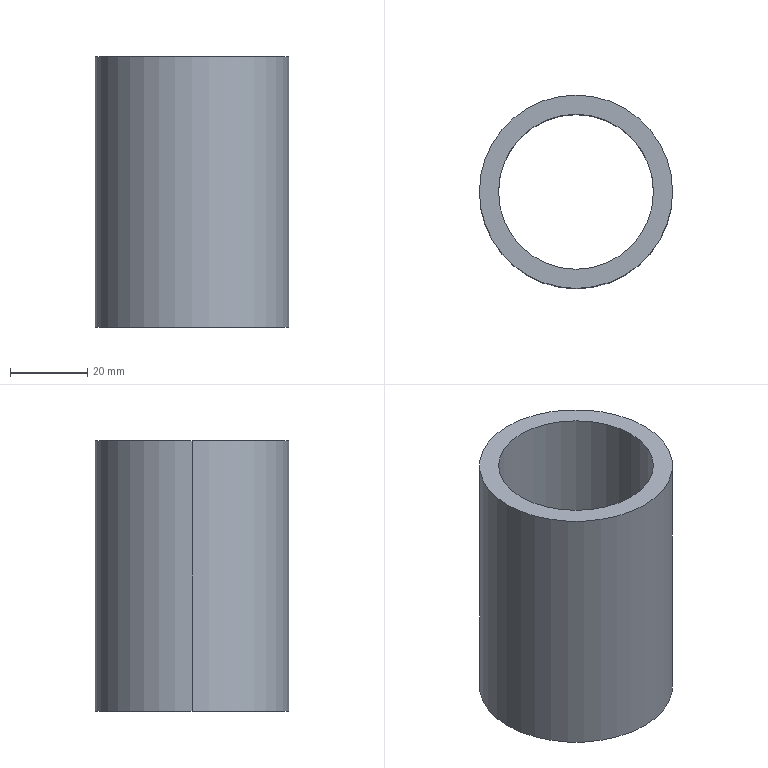Part | STEP file | LM-05-1230_default | 1 solid | 6 faces | box 50 x 50 x 70 mm | volume 49040 mm3 | cylinder 4 | plane 2 | commonest cylinder face diameters 40.1 x2 50 x2
STEP:
#1=CARTESIAN_POINT('',(0.,0.,0.));
#2=DIRECTION('',(0.,0.,1.));
#3=DIRECTION('',(1.,0.,0.));
#4=AXIS2_PLACEMENT_3D('',#1,#2,#3);
#5=CARTESIAN_POINT('',(-20.05,0.,35.));
#6=VERTEX_POINT('',#5);
#7=CARTESIAN_POINT('',(-20.05,0.,-35.));
#8=VERTEX_POINT('',#7);
#9=CARTESIAN_POINT('',(-20.05,0.,35.));
#10=DIRECTION('',(0.,0.,-1.));
#11=VECTOR('',#10,1.);
#12=LINE('',#9,#11);
#13=CARTESIAN_POINT('',(0.,0.,35.));
#14=DIRECTION('',(0.,0.,-1.));
#15=DIRECTION('',(-1.,0.,0.));
#16=AXIS2_PLACEMENT_3D('',#13,#14,#15);
#17=CYLINDRICAL_SURFACE('',#16,20.05);
#18=CARTESIAN_POINT('',(6.283,0.));
#19=DIRECTION('',(0.,1.));
#20=VECTOR('',#19,1.);
#21=LINE('',#18,#20);
#22=(GEOMETRIC_REPRESENTATION_CONTEXT(2)PARAMETRIC_REPRESENTATION_CONTEXT()REPRESENTATION_CONTEXT('',''));
#23=DEFINITIONAL_REPRESENTATION('',(#21),#22);
#24=PCURVE('',#17,#23);
#25=CARTESIAN_POINT('',(0.,0.,35.));
#26=DIRECTION('',(0.,0.,-1.));
#27=DIRECTION('',(-1.,0.,0.));
#28=AXIS2_PLACEMENT_3D('',#25,#26,#27);
#29=CYLINDRICAL_SURFACE('',#28,20.05);
#30=CARTESIAN_POINT('',(0.,0.));
#31=DIRECTION('',(0.,1.));
#32=VECTOR('',#31,1.);
#33=LINE('',#30,#32);
#34=(GEOMETRIC_REPRESENTATION_CONTEXT(2)PARAMETRIC_REPRESENTATION_CONTEXT()REPRESENTATION_CONTEXT('',''));
#35=DEFINITIONAL_REPRESENTATION('',(#33),#34);
#36=PCURVE('',#29,#35);
#37=SURFACE_CURVE('',#12,(#24,#36),.PCURVE_S1.);
#38=EDGE_CURVE('',#6,#8,#37,.T.);
#39=ORIENTED_EDGE('',*,*,#38,.T.);
#40=CARTESIAN_POINT('',(20.05,0.,-35.));
#41=VERTEX_POINT('',#40);
#42=CARTESIAN_POINT('',(0.,0.,-35.));
#43=DIRECTION('',(0.,0.,1.));
#44=DIRECTION('',(1.,0.,0.));
#45=AXIS2_PLACEMENT_3D('',#42,#43,#44);
#46=CIRCLE('',#45,20.05);
#47=CARTESIAN_POINT('',(9.425,70.));
#48=DIRECTION('',(-1.,0.));
#49=VECTOR('',#48,1.);
#50=LINE('',#47,#49);
#51=(GEOMETRIC_REPRESENTATION_CONTEXT(2)PARAMETRIC_REPRESENTATION_CONTEXT()REPRESENTATION_CONTEXT('',''));
#52=DEFINITIONAL_REPRESENTATION('',(#50),#51);
#53=PCURVE('',#17,#52);
#54=CARTESIAN_POINT('',(0.,0.,-35.));
#55=DIRECTION('',(0.,0.,1.));
#56=DIRECTION('',(1.,0.,0.));
#57=AXIS2_PLACEMENT_3D('',#54,#55,#56);
#58=PLANE('',#57);
#59=CARTESIAN_POINT('',(0.,0.));
#60=DIRECTION('',(1.,0.));
#61=AXIS2_PLACEMENT_2D('',#59,#60);
#62=CIRCLE('',#61,20.05);
#63=(GEOMETRIC_REPRESENTATION_CONTEXT(2)PARAMETRIC_REPRESENTATION_CONTEXT()REPRESENTATION_CONTEXT('',''));
#64=DEFINITIONAL_REPRESENTATION('',(#62),#63);
#65=PCURVE('',#58,#64);
#66=SURFACE_CURVE('',#46,(#53,#65),.PCURVE_S1.);
#67=EDGE_CURVE('',#8,#41,#66,.T.);
#68=ORIENTED_EDGE('',*,*,#67,.T.);
#69=CARTESIAN_POINT('',(20.05,0.,35.));
#70=VERTEX_POINT('',#69);
#71=CARTESIAN_POINT('',(20.05,0.,35.));
#72=DIRECTION('',(0.,0.,-1.));
#73=VECTOR('',#72,1.);
#74=LINE('',#71,#73);
#75=CARTESIAN_POINT('',(3.142,0.));
#76=DIRECTION('',(0.,1.));
#77=VECTOR('',#76,1.);
#78=LINE('',#75,#77);
#79=(GEOMETRIC_REPRESENTATION_CONTEXT(2)PARAMETRIC_REPRESENTATION_CONTEXT()REPRESENTATION_CONTEXT('',''));
#80=DEFINITIONAL_REPRESENTATION('',(#78),#79);
#81=PCURVE('',#17,#80);
#82=CARTESIAN_POINT('',(3.142,0.));
#83=DIRECTION('',(0.,1.));
#84=VECTOR('',#83,1.);
#85=LINE('',#82,#84);
#86=(GEOMETRIC_REPRESENTATION_CONTEXT(2)PARAMETRIC_REPRESENTATION_CONTEXT()REPRESENTATION_CONTEXT('',''));
#87=DEFINITIONAL_REPRESENTATION('',(#85),#86);
#88=PCURVE('',#29,#87);
#89=SURFACE_CURVE('',#74,(#81,#88),.PCURVE_S1.);
#90=EDGE_CURVE('',#70,#41,#89,.T.);
#91=ORIENTED_EDGE('',*,*,#90,.F.);
#92=CARTESIAN_POINT('',(0.,0.,35.));
#93=DIRECTION('',(0.,0.,1.));
#94=DIRECTION('',(1.,0.,0.));
#95=AXIS2_PLACEMENT_3D('',#92,#93,#94);
#96=CIRCLE('',#95,20.05);
#97=CARTESIAN_POINT('',(9.425,0.));
#98=DIRECTION('',(-1.,0.));
#99=VECTOR('',#98,1.);
#100=LINE('',#97,#99);
#101=(GEOMETRIC_REPRESENTATION_CONTEXT(2)PARAMETRIC_REPRESENTATION_CONTEXT()REPRESENTATION_CONTEXT('',''));
#102=DEFINITIONAL_REPRESENTATION('',(#100),#101);
#103=PCURVE('',#17,#102);
#104=CARTESIAN_POINT('',(0.,0.,35.));
#105=DIRECTION('',(0.,0.,1.));
#106=DIRECTION('',(1.,0.,0.));
#107=AXIS2_PLACEMENT_3D('',#104,#105,#106);
#108=PLANE('',#107);
#109=CARTESIAN_POINT('',(0.,0.));
#110=DIRECTION('',(1.,0.));
#111=AXIS2_PLACEMENT_2D('',#109,#110);
#112=CIRCLE('',#111,20.05);
#113=(GEOMETRIC_REPRESENTATION_CONTEXT(2)PARAMETRIC_REPRESENTATION_CONTEXT()REPRESENTATION_CONTEXT('',''));
#114=DEFINITIONAL_REPRESENTATION('',(#112),#113);
#115=PCURVE('',#108,#114);
#116=SURFACE_CURVE('',#96,(#103,#115),.PCURVE_S1.);
#117=EDGE_CURVE('',#6,#70,#116,.T.);
#118=ORIENTED_EDGE('',*,*,#117,.F.);
#119=EDGE_LOOP('',(#39,#68,#91,#118));
#120=FACE_BOUND('',#119,.F.);
#121=ADVANCED_FACE('',(#120),#17,.F.);
#122=CARTESIAN_POINT('',(25.,0.,35.));
#123=VERTEX_POINT('',#122);
#124=CARTESIAN_POINT('',(-25.,0.,35.));
#125=VERTEX_POINT('',#124);
#126=CARTESIAN_POINT('',(0.,0.,35.));
#127=DIRECTION('',(0.,0.,1.));
#128=DIRECTION('',(1.,0.,0.));
#129=AXIS2_PLACEMENT_3D('',#126,#127,#128);
#130=CIRCLE('',#129,25.);
#131=CARTESIAN_POINT('',(0.,0.,35.));
#132=DIRECTION('',(0.,0.,-1.));
#133=DIRECTION('',(-1.,0.,0.));
#134=AXIS2_PLACEMENT_3D('',#131,#132,#133);
#135=CYLINDRICAL_SURFACE('',#134,25.);
#136=CARTESIAN_POINT('',(3.142,0.));
#137=DIRECTION('',(-1.,0.));
#138=VECTOR('',#137,1.);
#139=LINE('',#136,#138);
#140=(GEOMETRIC_REPRESENTATION_CONTEXT(2)PARAMETRIC_REPRESENTATION_CONTEXT()REPRESENTATION_CONTEXT('',''));
#141=DEFINITIONAL_REPRESENTATION('',(#139),#140);
#142=PCURVE('',#135,#141);
#143=CARTESIAN_POINT('',(0.,0.));
#144=DIRECTION('',(1.,0.));
#145=AXIS2_PLACEMENT_2D('',#143,#144);
#146=CIRCLE('',#145,25.);
#147=(GEOMETRIC_REPRESENTATION_CONTEXT(2)PARAMETRIC_REPRESENTATION_CONTEXT()REPRESENTATION_CONTEXT('',''));
#148=DEFINITIONAL_REPRESENTATION('',(#146),#147);
#149=PCURVE('',#108,#148);
#150=SURFACE_CURVE('',#130,(#142,#149),.PCURVE_S1.);
#151=EDGE_CURVE('',#123,#125,#150,.T.);
#152=ORIENTED_EDGE('',*,*,#151,.F.);
#153=CARTESIAN_POINT('',(25.,0.,-35.));
#154=VERTEX_POINT('',#153);
#155=CARTESIAN_POINT('',(25.,0.,35.));
#156=DIRECTION('',(0.,0.,-1.));
#157=VECTOR('',#156,1.);
#158=LINE('',#155,#157);
#159=CARTESIAN_POINT('',(3.142,0.));
#160=DIRECTION('',(0.,1.));
#161=VECTOR('',#160,1.);
#162=LINE('',#159,#161);
#163=(GEOMETRIC_REPRESENTATION_CONTEXT(2)PARAMETRIC_REPRESENTATION_CONTEXT()REPRESENTATION_CONTEXT('',''));
#164=DEFINITIONAL_REPRESENTATION('',(#162),#163);
#165=PCURVE('',#135,#164);
#166=CARTESIAN_POINT('',(0.,0.,35.));
#167=DIRECTION('',(0.,0.,-1.));
#168=DIRECTION('',(-1.,0.,0.));
#169=AXIS2_PLACEMENT_3D('',#166,#167,#168);
#170=CYLINDRICAL_SURFACE('',#169,25.);
#171=CARTESIAN_POINT('',(3.142,0.));
#172=DIRECTION('',(0.,1.));
#173=VECTOR('',#172,1.);
#174=LINE('',#171,#173);
#175=(GEOMETRIC_REPRESENTATION_CONTEXT(2)PARAMETRIC_REPRESENTATION_CONTEXT()REPRESENTATION_CONTEXT('',''));
#176=DEFINITIONAL_REPRESENTATION('',(#174),#175);
#177=PCURVE('',#170,#176);
#178=SURFACE_CURVE('',#158,(#165,#177),.PCURVE_S1.);
#179=EDGE_CURVE('',#123,#154,#178,.T.);
#180=ORIENTED_EDGE('',*,*,#179,.T.);
#181=CARTESIAN_POINT('',(-25.,0.,-35.));
#182=VERTEX_POINT('',#181);
#183=CARTESIAN_POINT('',(0.,0.,-35.));
#184=DIRECTION('',(0.,0.,1.));
#185=DIRECTION('',(1.,0.,0.));
#186=AXIS2_PLACEMENT_3D('',#183,#184,#185);
#187=CIRCLE('',#186,25.);
#188=CARTESIAN_POINT('',(3.142,70.));
#189=DIRECTION('',(-1.,0.));
#190=VECTOR('',#189,1.);
#191=LINE('',#188,#190);
#192=(GEOMETRIC_REPRESENTATION_CONTEXT(2)PARAMETRIC_REPRESENTATION_CONTEXT()REPRESENTATION_CONTEXT('',''));
#193=DEFINITIONAL_REPRESENTATION('',(#191),#192);
#194=PCURVE('',#135,#193);
#195=CARTESIAN_POINT('',(0.,0.));
#196=DIRECTION('',(1.,0.));
#197=AXIS2_PLACEMENT_2D('',#195,#196);
#198=CIRCLE('',#197,25.);
#199=(GEOMETRIC_REPRESENTATION_CONTEXT(2)PARAMETRIC_REPRESENTATION_CONTEXT()REPRESENTATION_CONTEXT('',''));
#200=DEFINITIONAL_REPRESENTATION('',(#198),#199);
#201=PCURVE('',#58,#200);
#202=SURFACE_CURVE('',#187,(#194,#201),.PCURVE_S1.);
#203=EDGE_CURVE('',#154,#182,#202,.T.);
#204=ORIENTED_EDGE('',*,*,#203,.T.);
#205=CARTESIAN_POINT('',(-25.,0.,35.));
#206=DIRECTION('',(0.,0.,-1.));
#207=VECTOR('',#206,1.);
#208=LINE('',#205,#207);
#209=CARTESIAN_POINT('',(0.,0.));
#210=DIRECTION('',(0.,1.));
#211=VECTOR('',#210,1.);
#212=LINE('',#209,#211);
#213=(GEOMETRIC_REPRESENTATION_CONTEXT(2)PARAMETRIC_REPRESENTATION_CONTEXT()REPRESENTATION_CONTEXT('',''));
#214=DEFINITIONAL_REPRESENTATION('',(#212),#213);
#215=PCURVE('',#135,#214);
#216=CARTESIAN_POINT('',(6.283,0.));
#217=DIRECTION('',(0.,1.));
#218=VECTOR('',#217,1.);
#219=LINE('',#216,#218);
#220=(GEOMETRIC_REPRESENTATION_CONTEXT(2)PARAMETRIC_REPRESENTATION_CONTEXT()REPRESENTATION_CONTEXT('',''));
#221=DEFINITIONAL_REPRESENTATION('',(#219),#220);
#222=PCURVE('',#170,#221);
#223=SURFACE_CURVE('',#208,(#215,#222),.PCURVE_S1.);
#224=EDGE_CURVE('',#125,#182,#223,.T.);
#225=ORIENTED_EDGE('',*,*,#224,.F.);
#226=EDGE_LOOP('',(#152,#180,#204,#225));
#227=FACE_BOUND('',#226,.T.);
#228=ADVANCED_FACE('',(#227),#135,.T.);
#229=CARTESIAN_POINT('',(0.,0.,35.));
#230=DIRECTION('',(0.,0.,1.));
#231=DIRECTION('',(1.,0.,0.));
#232=AXIS2_PLACEMENT_3D('',#229,#230,#231);
#233=CIRCLE('',#232,25.);
#234=CARTESIAN_POINT('',(0.,0.));
#235=DIRECTION('',(1.,0.));
#236=AXIS2_PLACEMENT_2D('',#234,#235);
#237=CIRCLE('',#236,25.);
#238=(GEOMETRIC_REPRESENTATION_CONTEXT(2)PARAMETRIC_REPRESENTATION_CONTEXT()REPRESENTATION_CONTEXT('',''));
#239=DEFINITIONAL_REPRESENTATION('',(#237),#238);
#240=PCURVE('',#108,#239);
#241=CARTESIAN_POINT('',(9.425,0.));
#242=DIRECTION('',(-1.,0.));
#243=VECTOR('',#242,1.);
#244=LINE('',#241,#243);
#245=(GEOMETRIC_REPRESENTATION_CONTEXT(2)PARAMETRIC_REPRESENTATION_CONTEXT()REPRESENTATION_CONTEXT('',''));
#246=DEFINITIONAL_REPRESENTATION('',(#244),#245);
#247=PCURVE('',#170,#246);
#248=SURFACE_CURVE('',#233,(#240,#247),.PCURVE_S1.);
#249=EDGE_CURVE('',#125,#123,#248,.T.);
#250=ORIENTED_EDGE('',*,*,#249,.T.);
#251=ORIENTED_EDGE('',*,*,#151,.T.);
#252=EDGE_LOOP('',(#250,#251));
#253=FACE_BOUND('',#252,.T.);
#254=ORIENTED_EDGE('',*,*,#117,.F.);
#255=CARTESIAN_POINT('',(0.,0.,35.));
#256=DIRECTION('',(0.,0.,1.));
#257=DIRECTION('',(1.,0.,0.));
#258=AXIS2_PLACEMENT_3D('',#255,#256,#257);
#259=CIRCLE('',#258,20.05);
#260=CARTESIAN_POINT('',(0.,0.));
#261=DIRECTION('',(1.,0.));
#262=AXIS2_PLACEMENT_2D('',#260,#261);
#263=CIRCLE('',#262,20.05);
#264=(GEOMETRIC_REPRESENTATION_CONTEXT(2)PARAMETRIC_REPRESENTATION_CONTEXT()REPRESENTATION_CONTEXT('',''));
#265=DEFINITIONAL_REPRESENTATION('',(#263),#264);
#266=PCURVE('',#108,#265);
#267=CARTESIAN_POINT('',(3.142,0.));
#268=DIRECTION('',(-1.,0.));
#269=VECTOR('',#268,1.);
#270=LINE('',#267,#269);
#271=(GEOMETRIC_REPRESENTATION_CONTEXT(2)PARAMETRIC_REPRESENTATION_CONTEXT()REPRESENTATION_CONTEXT('',''));
#272=DEFINITIONAL_REPRESENTATION('',(#270),#271);
#273=PCURVE('',#29,#272);
#274=SURFACE_CURVE('',#259,(#266,#273),.PCURVE_S1.);
#275=EDGE_CURVE('',#70,#6,#274,.T.);
#276=ORIENTED_EDGE('',*,*,#275,.F.);
#277=EDGE_LOOP('',(#254,#276));
#278=FACE_BOUND('',#277,.T.);
#279=ADVANCED_FACE('',(#253,#278),#108,.T.);
#280=CARTESIAN_POINT('',(0.,0.,-35.));
#281=DIRECTION('',(0.,0.,1.));
#282=DIRECTION('',(1.,0.,0.));
#283=AXIS2_PLACEMENT_3D('',#280,#281,#282);
#284=CIRCLE('',#283,25.);
#285=CARTESIAN_POINT('',(0.,0.));
#286=DIRECTION('',(1.,0.));
#287=AXIS2_PLACEMENT_2D('',#285,#286);
#288=CIRCLE('',#287,25.);
#289=(GEOMETRIC_REPRESENTATION_CONTEXT(2)PARAMETRIC_REPRESENTATION_CONTEXT()REPRESENTATION_CONTEXT('',''));
#290=DEFINITIONAL_REPRESENTATION('',(#288),#289);
#291=PCURVE('',#58,#290);
#292=CARTESIAN_POINT('',(9.425,70.));
#293=DIRECTION('',(-1.,0.));
#294=VECTOR('',#293,1.);
#295=LINE('',#292,#294);
#296=(GEOMETRIC_REPRESENTATION_CONTEXT(2)PARAMETRIC_REPRESENTATION_CONTEXT()REPRESENTATION_CONTEXT('',''));
#297=DEFINITIONAL_REPRESENTATION('',(#295),#296);
#298=PCURVE('',#170,#297);
#299=SURFACE_CURVE('',#284,(#291,#298),.PCURVE_S1.);
#300=EDGE_CURVE('',#182,#154,#299,.T.);
#301=ORIENTED_EDGE('',*,*,#300,.F.);
#302=ORIENTED_EDGE('',*,*,#203,.F.);
#303=EDGE_LOOP('',(#301,#302));
#304=FACE_BOUND('',#303,.T.);
#305=ORIENTED_EDGE('',*,*,#67,.T.);
#306=CARTESIAN_POINT('',(0.,0.,-35.));
#307=DIRECTION('',(0.,0.,1.));
#308=DIRECTION('',(1.,0.,0.));
#309=AXIS2_PLACEMENT_3D('',#306,#307,#308);
#310=CIRCLE('',#309,20.05);
#311=CARTESIAN_POINT('',(0.,0.));
#312=DIRECTION('',(1.,0.));
#313=AXIS2_PLACEMENT_2D('',#311,#312);
#314=CIRCLE('',#313,20.05);
#315=(GEOMETRIC_REPRESENTATION_CONTEXT(2)PARAMETRIC_REPRESENTATION_CONTEXT()REPRESENTATION_CONTEXT('',''));
#316=DEFINITIONAL_REPRESENTATION('',(#314),#315);
#317=PCURVE('',#58,#316);
#318=CARTESIAN_POINT('',(3.142,70.));
#319=DIRECTION('',(-1.,0.));
#320=VECTOR('',#319,1.);
#321=LINE('',#318,#320);
#322=(GEOMETRIC_REPRESENTATION_CONTEXT(2)PARAMETRIC_REPRESENTATION_CONTEXT()REPRESENTATION_CONTEXT('',''));
#323=DEFINITIONAL_REPRESENTATION('',(#321),#322);
#324=PCURVE('',#29,#323);
#325=SURFACE_CURVE('',#310,(#317,#324),.PCURVE_S1.);
#326=EDGE_CURVE('',#41,#8,#325,.T.);
#327=ORIENTED_EDGE('',*,*,#326,.T.);
#328=EDGE_LOOP('',(#305,#327));
#329=FACE_BOUND('',#328,.T.);
#330=ADVANCED_FACE('',(#304,#329),#58,.F.);
#331=ORIENTED_EDGE('',*,*,#179,.F.);
#332=ORIENTED_EDGE('',*,*,#249,.F.);
#333=ORIENTED_EDGE('',*,*,#224,.T.);
#334=ORIENTED_EDGE('',*,*,#300,.T.);
#335=EDGE_LOOP('',(#331,#332,#333,#334));
#336=FACE_BOUND('',#335,.T.);
#337=ADVANCED_FACE('',(#336),#170,.T.);
#338=ORIENTED_EDGE('',*,*,#326,.T.);
#339=ORIENTED_EDGE('',*,*,#38,.F.);
#340=ORIENTED_EDGE('',*,*,#275,.F.);
#341=ORIENTED_EDGE('',*,*,#90,.T.);
#342=EDGE_LOOP('',(#338,#339,#340,#341));
#343=FACE_BOUND('',#342,.F.);
#344=ADVANCED_FACE('',(#343),#29,.F.);
#345=CLOSED_SHELL('',(#121,#228,#279,#330,#337,#344));
#346=MANIFOLD_SOLID_BREP('',#345);
#347=(LENGTH_UNIT()NAMED_UNIT(*)SI_UNIT(.MILLI.,.METRE.));
#348=UNCERTAINTY_MEASURE_WITH_UNIT(LENGTH_MEASURE(0.0000001),#347,'','');
#349=(NAMED_UNIT(*)PLANE_ANGLE_UNIT()SI_UNIT($,.RADIAN.));
#350=(NAMED_UNIT(*)SI_UNIT($,.STERADIAN.)SOLID_ANGLE_UNIT());
#351=(GEOMETRIC_REPRESENTATION_CONTEXT(3)GLOBAL_UNCERTAINTY_ASSIGNED_CONTEXT((#348))GLOBAL_UNIT_ASSIGNED_CONTEXT((#347,#349,#350))REPRESENTATION_CONTEXT('',''));
#352=ADVANCED_BREP_SHAPE_REPRESENTATION('',(#4,#346),#351);